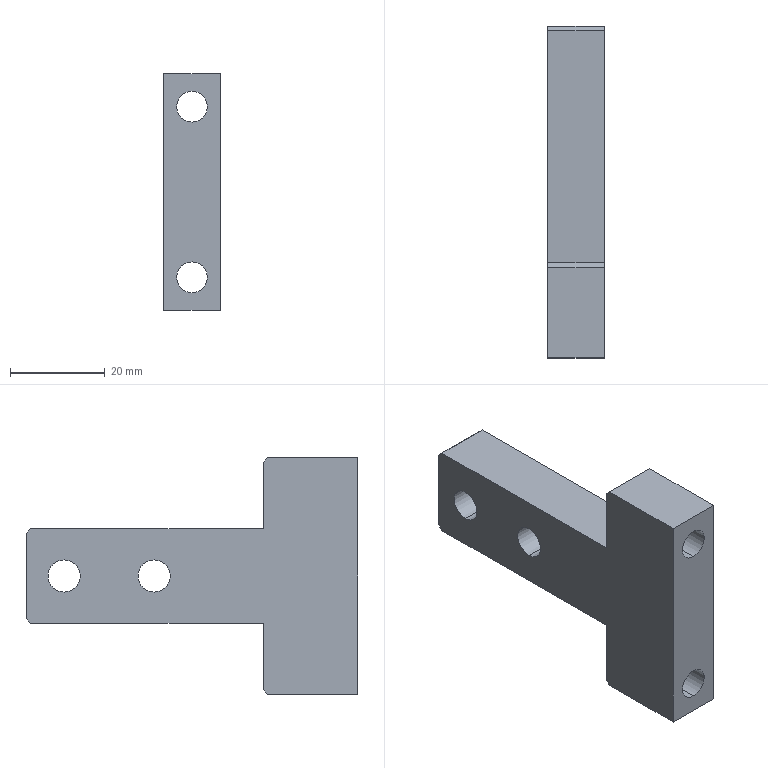Part | STEP file | 227H056256 Stop Block_Default | 1 solid | 22 faces | box 12 x 70 x 50 mm | volume 21777 mm3 | plane 14 | cylinder 8 | commonest cylinder face diameters 6.5 x4 6.8 x4